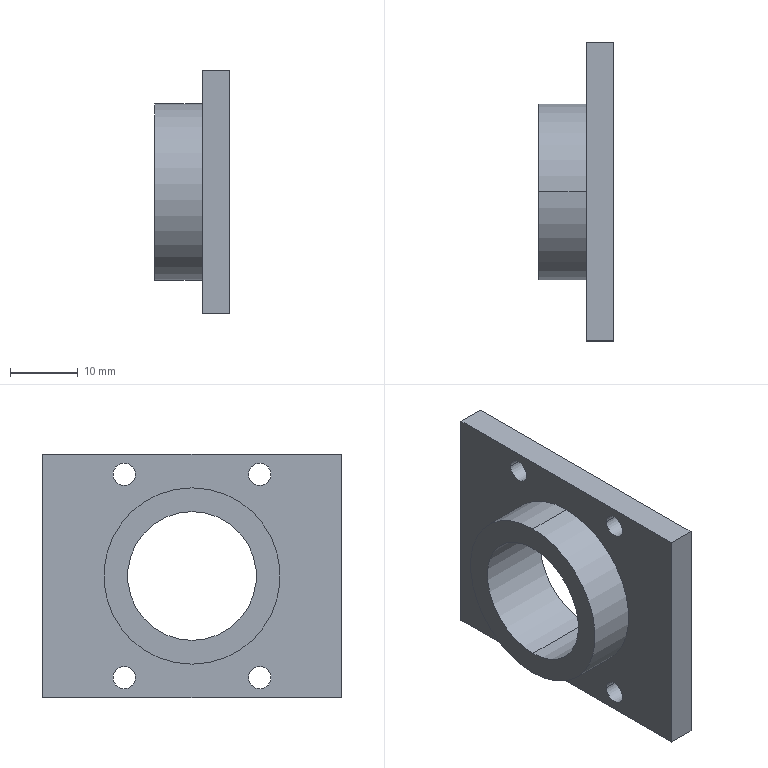Part | SolidWorks | features BaseBody 1 | 1 solid | 19 faces | box 11 x 44 x 36 mm | volume 6797 mm3 | cylinder 12 | plane 7 | commonest cylinder face diameters 3.3 x8 19 x2 26 x2
STEP:
#1=CARTESIAN_POINT('',(-2.,-11.65,33.));
#2=VERTEX_POINT('',#1);
#3=CARTESIAN_POINT('',(-2.,-8.35,33.));
#4=VERTEX_POINT('',#3);
#5=CARTESIAN_POINT('',(-2.,-10.,33.));
#6=DIRECTION('',(1.,0.,0.));
#7=DIRECTION('',(0.,1.,0.));
#8=AXIS2_PLACEMENT_3D('',#5,#6,#7);
#9=CIRCLE('',#8,1.65);
#10=EDGE_CURVE('',#2,#4,#9,.T.);
#11=ORIENTED_EDGE('',*,*,#10,.F.);
#12=CARTESIAN_POINT('',(2.,-11.65,33.));
#13=VERTEX_POINT('',#12);
#14=CARTESIAN_POINT('',(-14.2,-11.65,33.));
#15=DIRECTION('',(1.,0.,0.));
#16=VECTOR('',#15,1000.);
#17=LINE('',#14,#16);
#18=EDGE_CURVE('',#2,#13,#17,.T.);
#19=ORIENTED_EDGE('',*,*,#18,.T.);
#20=CARTESIAN_POINT('',(2.,-8.35,33.));
#21=VERTEX_POINT('',#20);
#22=CARTESIAN_POINT('',(2.,-10.,33.));
#23=DIRECTION('',(-1.,0.,0.));
#24=DIRECTION('',(0.,1.,0.));
#25=AXIS2_PLACEMENT_3D('',#22,#23,#24);
#26=CIRCLE('',#25,1.65);
#27=EDGE_CURVE('',#21,#13,#26,.T.);
#28=ORIENTED_EDGE('',*,*,#27,.F.);
#29=CARTESIAN_POINT('',(-14.2,-8.35,33.));
#30=DIRECTION('',(1.,0.,0.));
#31=VECTOR('',#30,1000.);
#32=LINE('',#29,#31);
#33=EDGE_CURVE('',#4,#21,#32,.T.);
#34=ORIENTED_EDGE('',*,*,#33,.F.);
#35=EDGE_LOOP('',(#11,#19,#28,#34));
#36=FACE_OUTER_BOUND('',#35,.T.);
#37=CARTESIAN_POINT('',(-14.2,-10.,33.));
#38=DIRECTION('',(1.,0.,0.));
#39=DIRECTION('',(0.,1.,0.));
#40=AXIS2_PLACEMENT_3D('',#37,#38,#39);
#41=CYLINDRICAL_SURFACE('',#40,1.65);
#42=ADVANCED_FACE('',(#36),#41,.F.);
#43=CARTESIAN_POINT('',(-9.,0.,27.5));
#44=VERTEX_POINT('',#43);
#45=CARTESIAN_POINT('',(-9.,0.,8.5));
#46=VERTEX_POINT('',#45);
#47=CARTESIAN_POINT('',(-9.,0.,18.));
#48=DIRECTION('',(1.,0.,0.));
#49=DIRECTION('',(0.,0.,-1.));
#50=AXIS2_PLACEMENT_3D('',#47,#48,#49);
#51=CIRCLE('',#50,9.5);
#52=EDGE_CURVE('',#44,#46,#51,.T.);
#53=ORIENTED_EDGE('',*,*,#52,.F.);
#54=CARTESIAN_POINT('',(2.,0.,27.5));
#55=VERTEX_POINT('',#54);
#56=CARTESIAN_POINT('',(-3.,0.,27.5));
#57=DIRECTION('',(1.,0.,0.));
#58=VECTOR('',#57,1000.);
#59=LINE('',#56,#58);
#60=EDGE_CURVE('',#44,#55,#59,.T.);
#61=ORIENTED_EDGE('',*,*,#60,.T.);
#62=CARTESIAN_POINT('',(2.,0.,8.5));
#63=VERTEX_POINT('',#62);
#64=CARTESIAN_POINT('',(2.,0.,18.));
#65=DIRECTION('',(-1.,0.,0.));
#66=DIRECTION('',(0.,0.,-1.));
#67=AXIS2_PLACEMENT_3D('',#64,#65,#66);
#68=CIRCLE('',#67,9.5);
#69=EDGE_CURVE('',#63,#55,#68,.T.);
#70=ORIENTED_EDGE('',*,*,#69,.F.);
#71=CARTESIAN_POINT('',(-3.,0.,8.5));
#72=DIRECTION('',(1.,0.,0.));
#73=VECTOR('',#72,1000.);
#74=LINE('',#71,#73);
#75=EDGE_CURVE('',#46,#63,#74,.T.);
#76=ORIENTED_EDGE('',*,*,#75,.F.);
#77=EDGE_LOOP('',(#53,#61,#70,#76));
#78=FACE_OUTER_BOUND('',#77,.T.);
#79=CARTESIAN_POINT('',(-3.,0.,18.));
#80=DIRECTION('',(1.,0.,0.));
#81=DIRECTION('',(0.,0.,-1.));
#82=AXIS2_PLACEMENT_3D('',#79,#80,#81);
#83=CYLINDRICAL_SURFACE('',#82,9.5);
#84=ADVANCED_FACE('',(#78),#83,.F.);
#85=CARTESIAN_POINT('',(-2.,-11.65,3.));
#86=VERTEX_POINT('',#85);
#87=CARTESIAN_POINT('',(-2.,-8.35,3.));
#88=VERTEX_POINT('',#87);
#89=CARTESIAN_POINT('',(-2.,-10.,3.));
#90=DIRECTION('',(1.,0.,0.));
#91=DIRECTION('',(0.,1.,0.));
#92=AXIS2_PLACEMENT_3D('',#89,#90,#91);
#93=CIRCLE('',#92,1.65);
#94=EDGE_CURVE('',#86,#88,#93,.T.);
#95=ORIENTED_EDGE('',*,*,#94,.F.);
#96=CARTESIAN_POINT('',(2.,-11.65,3.));
#97=VERTEX_POINT('',#96);
#98=CARTESIAN_POINT('',(-14.2,-11.65,3.));
#99=DIRECTION('',(1.,0.,0.));
#100=VECTOR('',#99,1000.);
#101=LINE('',#98,#100);
#102=EDGE_CURVE('',#86,#97,#101,.T.);
#103=ORIENTED_EDGE('',*,*,#102,.T.);
#104=CARTESIAN_POINT('',(2.,-8.35,3.));
#105=VERTEX_POINT('',#104);
#106=CARTESIAN_POINT('',(2.,-10.,3.));
#107=DIRECTION('',(-1.,0.,0.));
#108=DIRECTION('',(0.,1.,0.));
#109=AXIS2_PLACEMENT_3D('',#106,#107,#108);
#110=CIRCLE('',#109,1.65);
#111=EDGE_CURVE('',#105,#97,#110,.T.);
#112=ORIENTED_EDGE('',*,*,#111,.F.);
#113=CARTESIAN_POINT('',(-14.2,-8.35,3.));
#114=DIRECTION('',(1.,0.,0.));
#115=VECTOR('',#114,1000.);
#116=LINE('',#113,#115);
#117=EDGE_CURVE('',#88,#105,#116,.T.);
#118=ORIENTED_EDGE('',*,*,#117,.F.);
#119=EDGE_LOOP('',(#95,#103,#112,#118));
#120=FACE_OUTER_BOUND('',#119,.T.);
#121=CARTESIAN_POINT('',(-14.2,-10.,3.));
#122=DIRECTION('',(1.,0.,0.));
#123=DIRECTION('',(0.,1.,0.));
#124=AXIS2_PLACEMENT_3D('',#121,#122,#123);
#125=CYLINDRICAL_SURFACE('',#124,1.65);
#126=ADVANCED_FACE('',(#120),#125,.F.);
#127=CARTESIAN_POINT('',(-2.,8.35,33.));
#128=VERTEX_POINT('',#127);
#129=CARTESIAN_POINT('',(-2.,11.65,33.));
#130=VERTEX_POINT('',#129);
#131=CARTESIAN_POINT('',(-2.,10.,33.));
#132=DIRECTION('',(1.,0.,0.));
#133=DIRECTION('',(0.,1.,0.));
#134=AXIS2_PLACEMENT_3D('',#131,#132,#133);
#135=CIRCLE('',#134,1.65);
#136=EDGE_CURVE('',#128,#130,#135,.T.);
#137=ORIENTED_EDGE('',*,*,#136,.F.);
#138=CARTESIAN_POINT('',(2.,8.35,33.));
#139=VERTEX_POINT('',#138);
#140=CARTESIAN_POINT('',(-14.2,8.35,33.));
#141=DIRECTION('',(1.,0.,0.));
#142=VECTOR('',#141,1000.);
#143=LINE('',#140,#142);
#144=EDGE_CURVE('',#128,#139,#143,.T.);
#145=ORIENTED_EDGE('',*,*,#144,.T.);
#146=CARTESIAN_POINT('',(2.,11.65,33.));
#147=VERTEX_POINT('',#146);
#148=CARTESIAN_POINT('',(2.,10.,33.));
#149=DIRECTION('',(-1.,0.,0.));
#150=DIRECTION('',(0.,1.,0.));
#151=AXIS2_PLACEMENT_3D('',#148,#149,#150);
#152=CIRCLE('',#151,1.65);
#153=EDGE_CURVE('',#147,#139,#152,.T.);
#154=ORIENTED_EDGE('',*,*,#153,.F.);
#155=CARTESIAN_POINT('',(-14.2,11.65,33.));
#156=DIRECTION('',(1.,0.,0.));
#157=VECTOR('',#156,1000.);
#158=LINE('',#155,#157);
#159=EDGE_CURVE('',#130,#147,#158,.T.);
#160=ORIENTED_EDGE('',*,*,#159,.F.);
#161=EDGE_LOOP('',(#137,#145,#154,#160));
#162=FACE_OUTER_BOUND('',#161,.T.);
#163=CARTESIAN_POINT('',(-14.2,10.,33.));
#164=DIRECTION('',(1.,0.,0.));
#165=DIRECTION('',(0.,1.,0.));
#166=AXIS2_PLACEMENT_3D('',#163,#164,#165);
#167=CYLINDRICAL_SURFACE('',#166,1.65);
#168=ADVANCED_FACE('',(#162),#167,.F.);
#169=CARTESIAN_POINT('',(-2.,8.35,3.));
#170=VERTEX_POINT('',#169);
#171=CARTESIAN_POINT('',(-2.,11.65,3.));
#172=VERTEX_POINT('',#171);
#173=CARTESIAN_POINT('',(-2.,10.,3.));
#174=DIRECTION('',(1.,0.,0.));
#175=DIRECTION('',(0.,1.,0.));
#176=AXIS2_PLACEMENT_3D('',#173,#174,#175);
#177=CIRCLE('',#176,1.65);
#178=EDGE_CURVE('',#170,#172,#177,.T.);
#179=ORIENTED_EDGE('',*,*,#178,.F.);
#180=CARTESIAN_POINT('',(2.,8.35,3.));
#181=VERTEX_POINT('',#180);
#182=CARTESIAN_POINT('',(-14.2,8.35,3.));
#183=DIRECTION('',(1.,0.,0.));
#184=VECTOR('',#183,1000.);
#185=LINE('',#182,#184);
#186=EDGE_CURVE('',#170,#181,#185,.T.);
#187=ORIENTED_EDGE('',*,*,#186,.T.);
#188=CARTESIAN_POINT('',(2.,11.65,3.));
#189=VERTEX_POINT('',#188);
#190=CARTESIAN_POINT('',(2.,10.,3.));
#191=DIRECTION('',(-1.,0.,0.));
#192=DIRECTION('',(0.,1.,0.));
#193=AXIS2_PLACEMENT_3D('',#190,#191,#192);
#194=CIRCLE('',#193,1.65);
#195=EDGE_CURVE('',#189,#181,#194,.T.);
#196=ORIENTED_EDGE('',*,*,#195,.F.);
#197=CARTESIAN_POINT('',(-14.2,11.65,3.));
#198=DIRECTION('',(1.,0.,0.));
#199=VECTOR('',#198,1000.);
#200=LINE('',#197,#199);
#201=EDGE_CURVE('',#172,#189,#200,.T.);
#202=ORIENTED_EDGE('',*,*,#201,.F.);
#203=EDGE_LOOP('',(#179,#187,#196,#202));
#204=FACE_OUTER_BOUND('',#203,.T.);
#205=CARTESIAN_POINT('',(-14.2,10.,3.));
#206=DIRECTION('',(1.,0.,0.));
#207=DIRECTION('',(0.,1.,0.));
#208=AXIS2_PLACEMENT_3D('',#205,#206,#207);
#209=CYLINDRICAL_SURFACE('',#208,1.65);
#210=ADVANCED_FACE('',(#204),#209,.F.);
#211=CARTESIAN_POINT('',(-9.,0.,5.));
#212=VERTEX_POINT('',#211);
#213=CARTESIAN_POINT('',(-9.,0.,31.));
#214=VERTEX_POINT('',#213);
#215=CARTESIAN_POINT('',(-9.,0.,18.));
#216=DIRECTION('',(1.,0.,0.));
#217=DIRECTION('',(0.,0.,-1.));
#218=AXIS2_PLACEMENT_3D('',#215,#216,#217);
#219=CIRCLE('',#218,13.);
#220=EDGE_CURVE('',#212,#214,#219,.T.);
#221=ORIENTED_EDGE('',*,*,#220,.T.);
#222=CARTESIAN_POINT('',(-2.,0.,31.));
#223=VERTEX_POINT('',#222);
#224=CARTESIAN_POINT('',(-9.,0.,31.));
#225=DIRECTION('',(1.,0.,0.));
#226=VECTOR('',#225,1000.);
#227=LINE('',#224,#226);
#228=EDGE_CURVE('',#214,#223,#227,.T.);
#229=ORIENTED_EDGE('',*,*,#228,.T.);
#230=CARTESIAN_POINT('',(-2.,0.,5.));
#231=VERTEX_POINT('',#230);
#232=CARTESIAN_POINT('',(-2.,0.,18.));
#233=DIRECTION('',(-1.,0.,0.));
#234=DIRECTION('',(0.,0.,-1.));
#235=AXIS2_PLACEMENT_3D('',#232,#233,#234);
#236=CIRCLE('',#235,13.);
#237=EDGE_CURVE('',#223,#231,#236,.T.);
#238=ORIENTED_EDGE('',*,*,#237,.T.);
#239=CARTESIAN_POINT('',(-9.,0.,5.));
#240=DIRECTION('',(1.,0.,0.));
#241=VECTOR('',#240,1000.);
#242=LINE('',#239,#241);
#243=EDGE_CURVE('',#212,#231,#242,.T.);
#244=ORIENTED_EDGE('',*,*,#243,.F.);
#245=EDGE_LOOP('',(#221,#229,#238,#244));
#246=FACE_OUTER_BOUND('',#245,.T.);
#247=CARTESIAN_POINT('',(-9.,0.,18.));
#248=DIRECTION('',(1.,0.,0.));
#249=DIRECTION('',(0.,0.,-1.));
#250=AXIS2_PLACEMENT_3D('',#247,#248,#249);
#251=CYLINDRICAL_SURFACE('',#250,13.);
#252=ADVANCED_FACE('',(#246),#251,.T.);
#253=ORIENTED_EDGE('',*,*,#27,.T.);
#254=CARTESIAN_POINT('',(2.,-10.,33.));
#255=DIRECTION('',(-1.,0.,0.));
#256=DIRECTION('',(0.,1.,0.));
#257=AXIS2_PLACEMENT_3D('',#254,#255,#256);
#258=CIRCLE('',#257,1.65);
#259=EDGE_CURVE('',#13,#21,#258,.T.);
#260=ORIENTED_EDGE('',*,*,#259,.T.);
#261=EDGE_LOOP('',(#253,#260));
#262=FACE_BOUND('',#261,.T.);
#263=ORIENTED_EDGE('',*,*,#69,.T.);
#264=CARTESIAN_POINT('',(2.,0.,18.));
#265=DIRECTION('',(-1.,0.,0.));
#266=DIRECTION('',(0.,0.,-1.));
#267=AXIS2_PLACEMENT_3D('',#264,#265,#266);
#268=CIRCLE('',#267,9.5);
#269=EDGE_CURVE('',#55,#63,#268,.T.);
#270=ORIENTED_EDGE('',*,*,#269,.T.);
#271=EDGE_LOOP('',(#263,#270));
#272=FACE_BOUND('',#271,.T.);
#273=ORIENTED_EDGE('',*,*,#111,.T.);
#274=CARTESIAN_POINT('',(2.,-10.,3.));
#275=DIRECTION('',(-1.,0.,0.));
#276=DIRECTION('',(0.,1.,0.));
#277=AXIS2_PLACEMENT_3D('',#274,#275,#276);
#278=CIRCLE('',#277,1.65);
#279=EDGE_CURVE('',#97,#105,#278,.T.);
#280=ORIENTED_EDGE('',*,*,#279,.T.);
#281=EDGE_LOOP('',(#273,#280));
#282=FACE_BOUND('',#281,.T.);
#283=ORIENTED_EDGE('',*,*,#153,.T.);
#284=CARTESIAN_POINT('',(2.,10.,33.));
#285=DIRECTION('',(-1.,0.,0.));
#286=DIRECTION('',(0.,1.,0.));
#287=AXIS2_PLACEMENT_3D('',#284,#285,#286);
#288=CIRCLE('',#287,1.65);
#289=EDGE_CURVE('',#139,#147,#288,.T.);
#290=ORIENTED_EDGE('',*,*,#289,.T.);
#291=EDGE_LOOP('',(#283,#290));
#292=FACE_BOUND('',#291,.T.);
#293=ORIENTED_EDGE('',*,*,#195,.T.);
#294=CARTESIAN_POINT('',(2.,10.,3.));
#295=DIRECTION('',(-1.,0.,0.));
#296=DIRECTION('',(0.,1.,0.));
#297=AXIS2_PLACEMENT_3D('',#294,#295,#296);
#298=CIRCLE('',#297,1.65);
#299=EDGE_CURVE('',#181,#189,#298,.T.);
#300=ORIENTED_EDGE('',*,*,#299,.T.);
#301=EDGE_LOOP('',(#293,#300));
#302=FACE_BOUND('',#301,.T.);
#303=CARTESIAN_POINT('',(2.,22.,0.));
#304=VERTEX_POINT('',#303);
#305=CARTESIAN_POINT('',(2.,22.,36.));
#306=VERTEX_POINT('',#305);
#307=CARTESIAN_POINT('',(2.,22.,0.));
#308=DIRECTION('',(0.,0.,1.));
#309=VECTOR('',#308,1000.);
#310=LINE('',#307,#309);
#311=EDGE_CURVE('',#304,#306,#310,.T.);
#312=ORIENTED_EDGE('',*,*,#311,.T.);
#313=CARTESIAN_POINT('',(2.,-22.,36.));
#314=VERTEX_POINT('',#313);
#315=CARTESIAN_POINT('',(2.,-22.,36.));
#316=DIRECTION('',(0.,-1.,0.));
#317=VECTOR('',#316,1000.);
#318=LINE('',#315,#317);
#319=EDGE_CURVE('',#306,#314,#318,.T.);
#320=ORIENTED_EDGE('',*,*,#319,.T.);
#321=CARTESIAN_POINT('',(2.,-22.,0.));
#322=VERTEX_POINT('',#321);
#323=CARTESIAN_POINT('',(2.,-22.,0.));
#324=DIRECTION('',(0.,0.,-1.));
#325=VECTOR('',#324,1000.);
#326=LINE('',#323,#325);
#327=EDGE_CURVE('',#314,#322,#326,.T.);
#328=ORIENTED_EDGE('',*,*,#327,.T.);
#329=CARTESIAN_POINT('',(2.,-22.,0.));
#330=DIRECTION('',(0.,1.,0.));
#331=VECTOR('',#330,1000.);
#332=LINE('',#329,#331);
#333=EDGE_CURVE('',#322,#304,#332,.T.);
#334=ORIENTED_EDGE('',*,*,#333,.T.);
#335=EDGE_LOOP('',(#312,#320,#328,#334));
#336=FACE_OUTER_BOUND('',#335,.T.);
#337=CARTESIAN_POINT('',(2.,-22.,0.));
#338=DIRECTION('',(1.,0.,0.));
#339=DIRECTION('',(0.,0.,-1.));
#340=AXIS2_PLACEMENT_3D('',#337,#338,#339);
#341=PLANE('',#340);
#342=ADVANCED_FACE('',(#262,#272,#282,#292,#302,#336),#341,.T.);
#343=ORIENTED_EDGE('',*,*,#18,.F.);
#344=CARTESIAN_POINT('',(-2.,-10.,33.));
#345=DIRECTION('',(1.,0.,0.));
#346=DIRECTION('',(0.,1.,0.));
#347=AXIS2_PLACEMENT_3D('',#344,#345,#346);
#348=CIRCLE('',#347,1.65);
#349=EDGE_CURVE('',#4,#2,#348,.T.);
#350=ORIENTED_EDGE('',*,*,#349,.F.);
#351=ORIENTED_EDGE('',*,*,#33,.T.);
#352=ORIENTED_EDGE('',*,*,#259,.F.);
#353=EDGE_LOOP('',(#343,#350,#351,#352));
#354=FACE_OUTER_BOUND('',#353,.T.);
#355=CARTESIAN_POINT('',(-14.2,-10.,33.));
#356=DIRECTION('',(1.,0.,0.));
#357=DIRECTION('',(0.,1.,0.));
#358=AXIS2_PLACEMENT_3D('',#355,#356,#357);
#359=CYLINDRICAL_SURFACE('',#358,1.65);
#360=ADVANCED_FACE('',(#354),#359,.F.);
#361=ORIENTED_EDGE('',*,*,#60,.F.);
#362=CARTESIAN_POINT('',(-9.,0.,18.));
#363=DIRECTION('',(1.,0.,0.));
#364=DIRECTION('',(0.,0.,-1.));
#365=AXIS2_PLACEMENT_3D('',#362,#363,#364);
#366=CIRCLE('',#365,9.5);
#367=EDGE_CURVE('',#46,#44,#366,.T.);
#368=ORIENTED_EDGE('',*,*,#367,.F.);
#369=ORIENTED_EDGE('',*,*,#75,.T.);
#370=ORIENTED_EDGE('',*,*,#269,.F.);
#371=EDGE_LOOP('',(#361,#368,#369,#370));
#372=FACE_OUTER_BOUND('',#371,.T.);
#373=CARTESIAN_POINT('',(-3.,0.,18.));
#374=DIRECTION('',(1.,0.,0.));
#375=DIRECTION('',(0.,0.,-1.));
#376=AXIS2_PLACEMENT_3D('',#373,#374,#375);
#377=CYLINDRICAL_SURFACE('',#376,9.5);
#378=ADVANCED_FACE('',(#372),#377,.F.);
#379=ORIENTED_EDGE('',*,*,#102,.F.);
#380=CARTESIAN_POINT('',(-2.,-10.,3.));
#381=DIRECTION('',(1.,0.,0.));
#382=DIRECTION('',(0.,1.,0.));
#383=AXIS2_PLACEMENT_3D('',#380,#381,#382);
#384=CIRCLE('',#383,1.65);
#385=EDGE_CURVE('',#88,#86,#384,.T.);
#386=ORIENTED_EDGE('',*,*,#385,.F.);
#387=ORIENTED_EDGE('',*,*,#117,.T.);
#388=ORIENTED_EDGE('',*,*,#279,.F.);
#389=EDGE_LOOP('',(#379,#386,#387,#388));
#390=FACE_OUTER_BOUND('',#389,.T.);
#391=CARTESIAN_POINT('',(-14.2,-10.,3.));
#392=DIRECTION('',(1.,0.,0.));
#393=DIRECTION('',(0.,1.,0.));
#394=AXIS2_PLACEMENT_3D('',#391,#392,#393);
#395=CYLINDRICAL_SURFACE('',#394,1.65);
#396=ADVANCED_FACE('',(#390),#395,.F.);
#397=ORIENTED_EDGE('',*,*,#144,.F.);
#398=CARTESIAN_POINT('',(-2.,10.,33.));
#399=DIRECTION('',(1.,0.,0.));
#400=DIRECTION('',(0.,1.,0.));
#401=AXIS2_PLACEMENT_3D('',#398,#399,#400);
#402=CIRCLE('',#401,1.65);
#403=EDGE_CURVE('',#130,#128,#402,.T.);
#404=ORIENTED_EDGE('',*,*,#403,.F.);
#405=ORIENTED_EDGE('',*,*,#159,.T.);
#406=ORIENTED_EDGE('',*,*,#289,.F.);
#407=EDGE_LOOP('',(#397,#404,#405,#406));
#408=FACE_OUTER_BOUND('',#407,.T.);
#409=CARTESIAN_POINT('',(-14.2,10.,33.));
#410=DIRECTION('',(1.,0.,0.));
#411=DIRECTION('',(0.,1.,0.));
#412=AXIS2_PLACEMENT_3D('',#409,#410,#411);
#413=CYLINDRICAL_SURFACE('',#412,1.65);
#414=ADVANCED_FACE('',(#408),#413,.F.);
#415=ORIENTED_EDGE('',*,*,#186,.F.);
#416=CARTESIAN_POINT('',(-2.,10.,3.));
#417=DIRECTION('',(1.,0.,0.));
#418=DIRECTION('',(0.,1.,0.));
#419=AXIS2_PLACEMENT_3D('',#416,#417,#418);
#420=CIRCLE('',#419,1.65);
#421=EDGE_CURVE('',#172,#170,#420,.T.);
#422=ORIENTED_EDGE('',*,*,#421,.F.);
#423=ORIENTED_EDGE('',*,*,#201,.T.);
#424=ORIENTED_EDGE('',*,*,#299,.F.);
#425=EDGE_LOOP('',(#415,#422,#423,#424));
#426=FACE_OUTER_BOUND('',#425,.T.);
#427=CARTESIAN_POINT('',(-14.2,10.,3.));
#428=DIRECTION('',(1.,0.,0.));
#429=DIRECTION('',(0.,1.,0.));
#430=AXIS2_PLACEMENT_3D('',#427,#428,#429);
#431=CYLINDRICAL_SURFACE('',#430,1.65);
#432=ADVANCED_FACE('',(#426),#431,.F.);
#433=ORIENTED_EDGE('',*,*,#319,.F.);
#434=CARTESIAN_POINT('',(-2.,22.,36.));
#435=VERTEX_POINT('',#434);
#436=CARTESIAN_POINT('',(-2.,22.,36.));
#437=DIRECTION('',(-1.,0.,0.));
#438=VECTOR('',#437,1000.);
#439=LINE('',#436,#438);
#440=EDGE_CURVE('',#306,#435,#439,.T.);
#441=ORIENTED_EDGE('',*,*,#440,.T.);
#442=CARTESIAN_POINT('',(-2.,-22.,36.));
#443=VERTEX_POINT('',#442);
#444=CARTESIAN_POINT('',(-2.,-22.,36.));
#445=DIRECTION('',(0.,-1.,0.));
#446=VECTOR('',#445,1000.);
#447=LINE('',#444,#446);
#448=EDGE_CURVE('',#435,#443,#447,.T.);
#449=ORIENTED_EDGE('',*,*,#448,.T.);
#450=CARTESIAN_POINT('',(-2.,-22.,36.));
#451=DIRECTION('',(1.,0.,0.));
#452=VECTOR('',#451,1000.);
#453=LINE('',#450,#452);
#454=EDGE_CURVE('',#443,#314,#453,.T.);
#455=ORIENTED_EDGE('',*,*,#454,.T.);
#456=EDGE_LOOP('',(#433,#441,#449,#455));
#457=FACE_OUTER_BOUND('',#456,.T.);
#458=CARTESIAN_POINT('',(-2.,-22.,36.));
#459=DIRECTION('',(0.,0.,1.));
#460=DIRECTION('',(1.,0.,0.));
#461=AXIS2_PLACEMENT_3D('',#458,#459,#460);
#462=PLANE('',#461);
#463=ADVANCED_FACE('',(#457),#462,.T.);
#464=ORIENTED_EDGE('',*,*,#440,.F.);
#465=ORIENTED_EDGE('',*,*,#311,.F.);
#466=CARTESIAN_POINT('',(-2.,22.,0.));
#467=VERTEX_POINT('',#466);
#468=CARTESIAN_POINT('',(-2.,22.,0.));
#469=DIRECTION('',(-1.,0.,0.));
#470=VECTOR('',#469,1000.);
#471=LINE('',#468,#470);
#472=EDGE_CURVE('',#304,#467,#471,.T.);
#473=ORIENTED_EDGE('',*,*,#472,.T.);
#474=CARTESIAN_POINT('',(-2.,22.,0.));
#475=DIRECTION('',(0.,0.,1.));
#476=VECTOR('',#475,1000.);
#477=LINE('',#474,#476);
#478=EDGE_CURVE('',#467,#435,#477,.T.);
#479=ORIENTED_EDGE('',*,*,#478,.T.);
#480=EDGE_LOOP('',(#464,#465,#473,#479));
#481=FACE_OUTER_BOUND('',#480,.T.);
#482=CARTESIAN_POINT('',(-2.,22.,0.));
#483=DIRECTION('',(0.,1.,0.));
#484=DIRECTION('',(0.,0.,1.));
#485=AXIS2_PLACEMENT_3D('',#482,#483,#484);
#486=PLANE('',#485);
#487=ADVANCED_FACE('',(#481),#486,.T.);
#488=ORIENTED_EDGE('',*,*,#333,.F.);
#489=CARTESIAN_POINT('',(-2.,-22.,0.));
#490=VERTEX_POINT('',#489);
#491=CARTESIAN_POINT('',(-2.,-22.,0.));
#492=DIRECTION('',(1.,0.,0.));
#493=VECTOR('',#492,1000.);
#494=LINE('',#491,#493);
#495=EDGE_CURVE('',#490,#322,#494,.T.);
#496=ORIENTED_EDGE('',*,*,#495,.F.);
#497=CARTESIAN_POINT('',(-2.,-22.,0.));
#498=DIRECTION('',(0.,-1.,0.));
#499=VECTOR('',#498,1000.);
#500=LINE('',#497,#499);
#501=EDGE_CURVE('',#467,#490,#500,.T.);
#502=ORIENTED_EDGE('',*,*,#501,.F.);
#503=ORIENTED_EDGE('',*,*,#472,.F.);
#504=EDGE_LOOP('',(#488,#496,#502,#503));
#505=FACE_OUTER_BOUND('',#504,.T.);
#506=CARTESIAN_POINT('',(-2.,-22.,0.));
#507=DIRECTION('',(0.,0.,1.));
#508=DIRECTION('',(1.,0.,0.));
#509=AXIS2_PLACEMENT_3D('',#506,#507,#508);
#510=PLANE('',#509);
#511=ADVANCED_FACE('',(#505),#510,.F.);
#512=ORIENTED_EDGE('',*,*,#454,.F.);
#513=CARTESIAN_POINT('',(-2.,-22.,0.));
#514=DIRECTION('',(0.,0.,1.));
#515=VECTOR('',#514,1000.);
#516=LINE('',#513,#515);
#517=EDGE_CURVE('',#490,#443,#516,.T.);
#518=ORIENTED_EDGE('',*,*,#517,.F.);
#519=ORIENTED_EDGE('',*,*,#495,.T.);
#520=ORIENTED_EDGE('',*,*,#327,.F.);
#521=EDGE_LOOP('',(#512,#518,#519,#520));
#522=FACE_OUTER_BOUND('',#521,.T.);
#523=CARTESIAN_POINT('',(-2.,-22.,0.));
#524=DIRECTION('',(0.,1.,0.));
#525=DIRECTION('',(0.,0.,1.));
#526=AXIS2_PLACEMENT_3D('',#523,#524,#525);
#527=PLANE('',#526);
#528=ADVANCED_FACE('',(#522),#527,.F.);
#529=ORIENTED_EDGE('',*,*,#349,.T.);
#530=ORIENTED_EDGE('',*,*,#10,.T.);
#531=EDGE_LOOP('',(#529,#530));
#532=FACE_BOUND('',#531,.T.);
#533=CARTESIAN_POINT('',(-2.,0.,18.));
#534=DIRECTION('',(-1.,0.,0.));
#535=DIRECTION('',(0.,0.,-1.));
#536=AXIS2_PLACEMENT_3D('',#533,#534,#535);
#537=CIRCLE('',#536,13.);
#538=EDGE_CURVE('',#231,#223,#537,.T.);
#539=ORIENTED_EDGE('',*,*,#538,.F.);
#540=ORIENTED_EDGE('',*,*,#237,.F.);
#541=EDGE_LOOP('',(#539,#540));
#542=FACE_BOUND('',#541,.T.);
#543=ORIENTED_EDGE('',*,*,#385,.T.);
#544=ORIENTED_EDGE('',*,*,#94,.T.);
#545=EDGE_LOOP('',(#543,#544));
#546=FACE_BOUND('',#545,.T.);
#547=ORIENTED_EDGE('',*,*,#403,.T.);
#548=ORIENTED_EDGE('',*,*,#136,.T.);
#549=EDGE_LOOP('',(#547,#548));
#550=FACE_BOUND('',#549,.T.);
#551=ORIENTED_EDGE('',*,*,#421,.T.);
#552=ORIENTED_EDGE('',*,*,#178,.T.);
#553=EDGE_LOOP('',(#551,#552));
#554=FACE_BOUND('',#553,.T.);
#555=ORIENTED_EDGE('',*,*,#478,.F.);
#556=ORIENTED_EDGE('',*,*,#501,.T.);
#557=ORIENTED_EDGE('',*,*,#517,.T.);
#558=ORIENTED_EDGE('',*,*,#448,.F.);
#559=EDGE_LOOP('',(#555,#556,#557,#558));
#560=FACE_OUTER_BOUND('',#559,.T.);
#561=CARTESIAN_POINT('',(-2.,-22.,0.));
#562=DIRECTION('',(1.,0.,0.));
#563=DIRECTION('',(0.,0.,-1.));
#564=AXIS2_PLACEMENT_3D('',#561,#562,#563);
#565=PLANE('',#564);
#566=ADVANCED_FACE('',(#532,#542,#546,#550,#554,#560),#565,.F.);
#567=ORIENTED_EDGE('',*,*,#367,.T.);
#568=ORIENTED_EDGE('',*,*,#52,.T.);
#569=EDGE_LOOP('',(#567,#568));
#570=FACE_BOUND('',#569,.T.);
#571=ORIENTED_EDGE('',*,*,#220,.F.);
#572=CARTESIAN_POINT('',(-9.,0.,18.));
#573=DIRECTION('',(1.,0.,0.));
#574=DIRECTION('',(0.,0.,-1.));
#575=AXIS2_PLACEMENT_3D('',#572,#573,#574);
#576=CIRCLE('',#575,13.);
#577=EDGE_CURVE('',#214,#212,#576,.T.);
#578=ORIENTED_EDGE('',*,*,#577,.F.);
#579=EDGE_LOOP('',(#571,#578));
#580=FACE_OUTER_BOUND('',#579,.T.);
#581=CARTESIAN_POINT('',(-9.,0.,18.));
#582=DIRECTION('',(1.,0.,0.));
#583=DIRECTION('',(0.,0.,-1.));
#584=AXIS2_PLACEMENT_3D('',#581,#582,#583);
#585=PLANE('',#584);
#586=ADVANCED_FACE('',(#570,#580),#585,.F.);
#587=ORIENTED_EDGE('',*,*,#228,.F.);
#588=ORIENTED_EDGE('',*,*,#577,.T.);
#589=ORIENTED_EDGE('',*,*,#243,.T.);
#590=ORIENTED_EDGE('',*,*,#538,.T.);
#591=EDGE_LOOP('',(#587,#588,#589,#590));
#592=FACE_OUTER_BOUND('',#591,.T.);
#593=CARTESIAN_POINT('',(-9.,0.,18.));
#594=DIRECTION('',(1.,0.,0.));
#595=DIRECTION('',(0.,0.,-1.));
#596=AXIS2_PLACEMENT_3D('',#593,#594,#595);
#597=CYLINDRICAL_SURFACE('',#596,13.);
#598=ADVANCED_FACE('',(#592),#597,.T.);
#599=CLOSED_SHELL('',(#42,#84,#126,#168,#210,#252,#342,#360,#378,#396,#414,#432,#463,#487,#511,#528,#566,#586,#598));
#600=MANIFOLD_SOLID_BREP('',#599);
#601=CARTESIAN_POINT('',(0.,0.,0.));
#602=DIRECTION('',(0.,0.,1.));
#603=DIRECTION('',(1.,0.,0.));
#604=AXIS2_PLACEMENT_3D('',#601,#602,#603);
#605=(LENGTH_UNIT()NAMED_UNIT(*)SI_UNIT(.MILLI.,.METRE.));
#606=UNCERTAINTY_MEASURE_WITH_UNIT(LENGTH_MEASURE(0.00001),#605,'','');
#607=(NAMED_UNIT(*)PLANE_ANGLE_UNIT()SI_UNIT($,.RADIAN.));
#608=(NAMED_UNIT(*)SI_UNIT($,.STERADIAN.)SOLID_ANGLE_UNIT());
#609=(GEOMETRIC_REPRESENTATION_CONTEXT(3)GLOBAL_UNCERTAINTY_ASSIGNED_CONTEXT((#606))GLOBAL_UNIT_ASSIGNED_CONTEXT((#605,#607,#608))REPRESENTATION_CONTEXT('',''));
#610=ADVANCED_BREP_SHAPE_REPRESENTATION('',(#600,#604),#609);